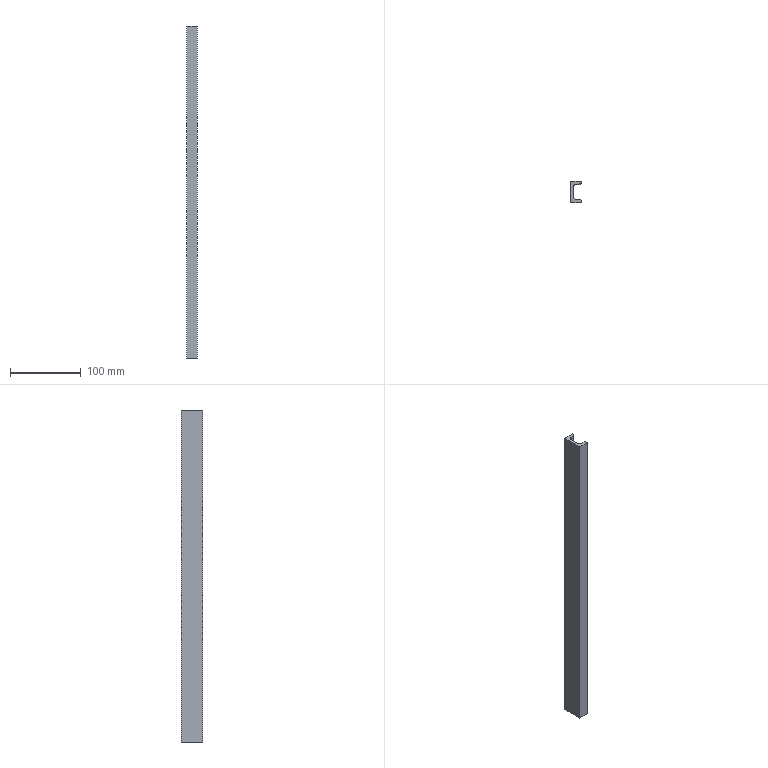Part | STEP file | DIN 1026-1 U 30x15 1785507675323 | 1 solid | 14 faces | box 15 x 30 x 470 mm | volume 103990 mm3 | plane 10 | cylinder 4 | commonest cylinder face diameters 4 x2 9 x2
STEP:
#1=CARTESIAN_POINT('',(4.,-6.066,485.));
#2=VERTEX_POINT('',#1);
#3=CARTESIAN_POINT('',(8.141,-10.551,485.));
#4=VERTEX_POINT('',#3);
#5=CARTESIAN_POINT('',(8.5,-6.066,485.));
#6=DIRECTION('',(0.,0.,1.));
#7=DIRECTION('',(-1.,0.,0.));
#8=AXIS2_PLACEMENT_3D('',#5,#6,#7);
#9=CIRCLE('',#8,4.5);
#10=EDGE_CURVE('',#2,#4,#9,.T.);
#11=ORIENTED_EDGE('',*,*,#10,.T.);
#12=CARTESIAN_POINT('',(8.141,-10.551,15.));
#13=VERTEX_POINT('',#12);
#14=CARTESIAN_POINT('',(8.141,-10.551,0.));
#15=DIRECTION('',(0.,0.,1.));
#16=VECTOR('',#15,10.);
#17=LINE('',#14,#16);
#18=EDGE_CURVE('',#13,#4,#17,.T.);
#19=ORIENTED_EDGE('',*,*,#18,.F.);
#20=CARTESIAN_POINT('',(4.,-6.066,15.));
#21=VERTEX_POINT('',#20);
#22=CARTESIAN_POINT('',(8.5,-6.066,15.));
#23=DIRECTION('',(0.,0.,1.));
#24=DIRECTION('',(-1.,0.,0.));
#25=AXIS2_PLACEMENT_3D('',#22,#23,#24);
#26=CIRCLE('',#25,4.5);
#27=EDGE_CURVE('',#21,#13,#26,.T.);
#28=ORIENTED_EDGE('',*,*,#27,.F.);
#29=CARTESIAN_POINT('',(4.,-6.066,0.));
#30=DIRECTION('',(0.,0.,1.));
#31=VECTOR('',#30,10.);
#32=LINE('',#29,#31);
#33=EDGE_CURVE('',#21,#2,#32,.T.);
#34=ORIENTED_EDGE('',*,*,#33,.T.);
#35=EDGE_LOOP('',(#11,#19,#28,#34));
#36=FACE_OUTER_BOUND('',#35,.T.);
#37=CARTESIAN_POINT('',(8.5,-6.066,0.));
#38=DIRECTION('',(0.,0.,1.));
#39=DIRECTION('',(-1.,0.,0.));
#40=AXIS2_PLACEMENT_3D('',#37,#38,#39);
#41=CYLINDRICAL_SURFACE('',#40,4.5);
#42=ADVANCED_FACE('',(#36),#41,.F.);
#43=CARTESIAN_POINT('',(13.159,-10.953,485.));
#44=VERTEX_POINT('',#43);
#45=CARTESIAN_POINT('',(7.403,-10.492,485.));
#46=DIRECTION('',(0.9968,-0.07975,0.));
#47=VECTOR('',#46,10.);
#48=LINE('',#45,#47);
#49=EDGE_CURVE('',#4,#44,#48,.T.);
#50=ORIENTED_EDGE('',*,*,#49,.T.);
#51=CARTESIAN_POINT('',(13.159,-10.953,15.));
#52=VERTEX_POINT('',#51);
#53=CARTESIAN_POINT('',(13.159,-10.953,0.));
#54=DIRECTION('',(0.,0.,1.));
#55=VECTOR('',#54,10.);
#56=LINE('',#53,#55);
#57=EDGE_CURVE('',#52,#44,#56,.T.);
#58=ORIENTED_EDGE('',*,*,#57,.F.);
#59=CARTESIAN_POINT('',(7.403,-10.492,15.));
#60=DIRECTION('',(0.9968,-0.07975,0.));
#61=VECTOR('',#60,10.);
#62=LINE('',#59,#61);
#63=EDGE_CURVE('',#13,#52,#62,.T.);
#64=ORIENTED_EDGE('',*,*,#63,.F.);
#65=ORIENTED_EDGE('',*,*,#18,.T.);
#66=EDGE_LOOP('',(#50,#58,#64,#65));
#67=FACE_OUTER_BOUND('',#66,.T.);
#68=CARTESIAN_POINT('',(8.141,-10.551,0.));
#69=DIRECTION('',(0.07975,0.9968,0.));
#70=DIRECTION('',(0.,0.,1.));
#71=AXIS2_PLACEMENT_3D('',#68,#69,#70);
#72=PLANE('',#71);
#73=ADVANCED_FACE('',(#67),#72,.T.);
#74=CARTESIAN_POINT('',(15.,-12.946,485.));
#75=VERTEX_POINT('',#74);
#76=CARTESIAN_POINT('',(13.,-12.946,485.));
#77=DIRECTION('',(0.,0.,-1.));
#78=DIRECTION('',(-1.,0.,0.));
#79=AXIS2_PLACEMENT_3D('',#76,#77,#78);
#80=CIRCLE('',#79,2.);
#81=EDGE_CURVE('',#44,#75,#80,.T.);
#82=ORIENTED_EDGE('',*,*,#81,.T.);
#83=CARTESIAN_POINT('',(15.,-12.946,15.));
#84=VERTEX_POINT('',#83);
#85=CARTESIAN_POINT('',(15.,-12.946,0.));
#86=DIRECTION('',(0.,0.,1.));
#87=VECTOR('',#86,10.);
#88=LINE('',#85,#87);
#89=EDGE_CURVE('',#84,#75,#88,.T.);
#90=ORIENTED_EDGE('',*,*,#89,.F.);
#91=CARTESIAN_POINT('',(13.,-12.946,15.));
#92=DIRECTION('',(0.,0.,-1.));
#93=DIRECTION('',(-1.,0.,0.));
#94=AXIS2_PLACEMENT_3D('',#91,#92,#93);
#95=CIRCLE('',#94,2.);
#96=EDGE_CURVE('',#52,#84,#95,.T.);
#97=ORIENTED_EDGE('',*,*,#96,.F.);
#98=ORIENTED_EDGE('',*,*,#57,.T.);
#99=EDGE_LOOP('',(#82,#90,#97,#98));
#100=FACE_OUTER_BOUND('',#99,.T.);
#101=CARTESIAN_POINT('',(13.,-12.946,0.));
#102=DIRECTION('',(0.,0.,1.));
#103=DIRECTION('',(-1.,0.,0.));
#104=AXIS2_PLACEMENT_3D('',#101,#102,#103);
#105=CYLINDRICAL_SURFACE('',#104,2.);
#106=ADVANCED_FACE('',(#100),#105,.T.);
#107=CARTESIAN_POINT('',(15.,-15.,485.));
#108=VERTEX_POINT('',#107);
#109=CARTESIAN_POINT('',(15.,-6.473,485.));
#110=DIRECTION('',(0.,-1.,0.));
#111=VECTOR('',#110,10.);
#112=LINE('',#109,#111);
#113=EDGE_CURVE('',#75,#108,#112,.T.);
#114=ORIENTED_EDGE('',*,*,#113,.T.);
#115=CARTESIAN_POINT('',(15.,-15.,15.));
#116=VERTEX_POINT('',#115);
#117=CARTESIAN_POINT('',(15.,-15.,0.));
#118=DIRECTION('',(0.,0.,1.));
#119=VECTOR('',#118,10.);
#120=LINE('',#117,#119);
#121=EDGE_CURVE('',#116,#108,#120,.T.);
#122=ORIENTED_EDGE('',*,*,#121,.F.);
#123=CARTESIAN_POINT('',(15.,-6.473,15.));
#124=DIRECTION('',(0.,-1.,0.));
#125=VECTOR('',#124,10.);
#126=LINE('',#123,#125);
#127=EDGE_CURVE('',#84,#116,#126,.T.);
#128=ORIENTED_EDGE('',*,*,#127,.F.);
#129=ORIENTED_EDGE('',*,*,#89,.T.);
#130=EDGE_LOOP('',(#114,#122,#128,#129));
#131=FACE_OUTER_BOUND('',#130,.T.);
#132=CARTESIAN_POINT('',(15.,-12.946,0.));
#133=DIRECTION('',(1.,0.,0.));
#134=DIRECTION('',(0.,0.,-1.));
#135=AXIS2_PLACEMENT_3D('',#132,#133,#134);
#136=PLANE('',#135);
#137=ADVANCED_FACE('',(#131),#136,.T.);
#138=CARTESIAN_POINT('',(0.,-15.,485.));
#139=VERTEX_POINT('',#138);
#140=CARTESIAN_POINT('',(11.25,-15.,485.));
#141=DIRECTION('',(-1.,0.,0.));
#142=VECTOR('',#141,10.);
#143=LINE('',#140,#142);
#144=EDGE_CURVE('',#108,#139,#143,.T.);
#145=ORIENTED_EDGE('',*,*,#144,.T.);
#146=CARTESIAN_POINT('',(0.,-15.,15.));
#147=VERTEX_POINT('',#146);
#148=CARTESIAN_POINT('',(0.,-15.,0.));
#149=DIRECTION('',(0.,0.,1.));
#150=VECTOR('',#149,10.);
#151=LINE('',#148,#150);
#152=EDGE_CURVE('',#147,#139,#151,.T.);
#153=ORIENTED_EDGE('',*,*,#152,.F.);
#154=CARTESIAN_POINT('',(11.25,-15.,15.));
#155=DIRECTION('',(-1.,0.,0.));
#156=VECTOR('',#155,10.);
#157=LINE('',#154,#156);
#158=EDGE_CURVE('',#116,#147,#157,.T.);
#159=ORIENTED_EDGE('',*,*,#158,.F.);
#160=ORIENTED_EDGE('',*,*,#121,.T.);
#161=EDGE_LOOP('',(#145,#153,#159,#160));
#162=FACE_OUTER_BOUND('',#161,.T.);
#163=CARTESIAN_POINT('',(15.,-15.,0.));
#164=DIRECTION('',(0.,-1.,0.));
#165=DIRECTION('',(0.,0.,-1.));
#166=AXIS2_PLACEMENT_3D('',#163,#164,#165);
#167=PLANE('',#166);
#168=ADVANCED_FACE('',(#162),#167,.T.);
#169=CARTESIAN_POINT('',(0.,15.,485.));
#170=VERTEX_POINT('',#169);
#171=CARTESIAN_POINT('',(0.,0.,485.));
#172=DIRECTION('',(0.,1.,0.));
#173=VECTOR('',#172,10.);
#174=LINE('',#171,#173);
#175=EDGE_CURVE('',#139,#170,#174,.T.);
#176=ORIENTED_EDGE('',*,*,#175,.T.);
#177=CARTESIAN_POINT('',(0.,15.,15.));
#178=VERTEX_POINT('',#177);
#179=CARTESIAN_POINT('',(0.,15.,0.));
#180=DIRECTION('',(0.,0.,1.));
#181=VECTOR('',#180,10.);
#182=LINE('',#179,#181);
#183=EDGE_CURVE('',#178,#170,#182,.T.);
#184=ORIENTED_EDGE('',*,*,#183,.F.);
#185=CARTESIAN_POINT('',(0.,0.,15.));
#186=DIRECTION('',(0.,1.,0.));
#187=VECTOR('',#186,10.);
#188=LINE('',#185,#187);
#189=EDGE_CURVE('',#147,#178,#188,.T.);
#190=ORIENTED_EDGE('',*,*,#189,.F.);
#191=ORIENTED_EDGE('',*,*,#152,.T.);
#192=EDGE_LOOP('',(#176,#184,#190,#191));
#193=FACE_OUTER_BOUND('',#192,.T.);
#194=CARTESIAN_POINT('',(0.,0.,0.));
#195=DIRECTION('',(-1.,0.,0.));
#196=DIRECTION('',(0.,0.,1.));
#197=AXIS2_PLACEMENT_3D('',#194,#195,#196);
#198=PLANE('',#197);
#199=ADVANCED_FACE('',(#193),#198,.T.);
#200=CARTESIAN_POINT('',(15.,15.,485.));
#201=VERTEX_POINT('',#200);
#202=CARTESIAN_POINT('',(3.75,15.,485.));
#203=DIRECTION('',(1.,0.,0.));
#204=VECTOR('',#203,10.);
#205=LINE('',#202,#204);
#206=EDGE_CURVE('',#170,#201,#205,.T.);
#207=ORIENTED_EDGE('',*,*,#206,.T.);
#208=CARTESIAN_POINT('',(15.,15.,15.));
#209=VERTEX_POINT('',#208);
#210=CARTESIAN_POINT('',(15.,15.,0.));
#211=DIRECTION('',(0.,0.,1.));
#212=VECTOR('',#211,10.);
#213=LINE('',#210,#212);
#214=EDGE_CURVE('',#209,#201,#213,.T.);
#215=ORIENTED_EDGE('',*,*,#214,.F.);
#216=CARTESIAN_POINT('',(3.75,15.,15.));
#217=DIRECTION('',(1.,0.,0.));
#218=VECTOR('',#217,10.);
#219=LINE('',#216,#218);
#220=EDGE_CURVE('',#178,#209,#219,.T.);
#221=ORIENTED_EDGE('',*,*,#220,.F.);
#222=ORIENTED_EDGE('',*,*,#183,.T.);
#223=EDGE_LOOP('',(#207,#215,#221,#222));
#224=FACE_OUTER_BOUND('',#223,.T.);
#225=CARTESIAN_POINT('',(0.,15.,0.));
#226=DIRECTION('',(0.,1.,0.));
#227=DIRECTION('',(0.,0.,1.));
#228=AXIS2_PLACEMENT_3D('',#225,#226,#227);
#229=PLANE('',#228);
#230=ADVANCED_FACE('',(#224),#229,.T.);
#231=CARTESIAN_POINT('',(15.,12.946,485.));
#232=VERTEX_POINT('',#231);
#233=CARTESIAN_POINT('',(15.,7.5,485.));
#234=DIRECTION('',(0.,-1.,0.));
#235=VECTOR('',#234,10.);
#236=LINE('',#233,#235);
#237=EDGE_CURVE('',#201,#232,#236,.T.);
#238=ORIENTED_EDGE('',*,*,#237,.T.);
#239=CARTESIAN_POINT('',(15.,12.946,15.));
#240=VERTEX_POINT('',#239);
#241=CARTESIAN_POINT('',(15.,12.946,0.));
#242=DIRECTION('',(0.,0.,1.));
#243=VECTOR('',#242,10.);
#244=LINE('',#241,#243);
#245=EDGE_CURVE('',#240,#232,#244,.T.);
#246=ORIENTED_EDGE('',*,*,#245,.F.);
#247=CARTESIAN_POINT('',(15.,7.5,15.));
#248=DIRECTION('',(0.,-1.,0.));
#249=VECTOR('',#248,10.);
#250=LINE('',#247,#249);
#251=EDGE_CURVE('',#209,#240,#250,.T.);
#252=ORIENTED_EDGE('',*,*,#251,.F.);
#253=ORIENTED_EDGE('',*,*,#214,.T.);
#254=EDGE_LOOP('',(#238,#246,#252,#253));
#255=FACE_OUTER_BOUND('',#254,.T.);
#256=CARTESIAN_POINT('',(15.,15.,0.));
#257=DIRECTION('',(1.,0.,0.));
#258=DIRECTION('',(0.,0.,-1.));
#259=AXIS2_PLACEMENT_3D('',#256,#257,#258);
#260=PLANE('',#259);
#261=ADVANCED_FACE('',(#255),#260,.T.);
#262=CARTESIAN_POINT('',(13.159,10.953,485.));
#263=VERTEX_POINT('',#262);
#264=CARTESIAN_POINT('',(13.,12.946,485.));
#265=DIRECTION('',(0.,0.,-1.));
#266=DIRECTION('',(-0.07975,0.9968,0.));
#267=AXIS2_PLACEMENT_3D('',#264,#265,#266);
#268=CIRCLE('',#267,2.);
#269=EDGE_CURVE('',#232,#263,#268,.T.);
#270=ORIENTED_EDGE('',*,*,#269,.T.);
#271=CARTESIAN_POINT('',(13.159,10.953,15.));
#272=VERTEX_POINT('',#271);
#273=CARTESIAN_POINT('',(13.159,10.953,0.));
#274=DIRECTION('',(0.,0.,1.));
#275=VECTOR('',#274,10.);
#276=LINE('',#273,#275);
#277=EDGE_CURVE('',#272,#263,#276,.T.);
#278=ORIENTED_EDGE('',*,*,#277,.F.);
#279=CARTESIAN_POINT('',(13.,12.946,15.));
#280=DIRECTION('',(0.,0.,-1.));
#281=DIRECTION('',(-0.07975,0.9968,0.));
#282=AXIS2_PLACEMENT_3D('',#279,#280,#281);
#283=CIRCLE('',#282,2.);
#284=EDGE_CURVE('',#240,#272,#283,.T.);
#285=ORIENTED_EDGE('',*,*,#284,.F.);
#286=ORIENTED_EDGE('',*,*,#245,.T.);
#287=EDGE_LOOP('',(#270,#278,#285,#286));
#288=FACE_OUTER_BOUND('',#287,.T.);
#289=CARTESIAN_POINT('',(13.,12.946,0.));
#290=DIRECTION('',(0.,0.,1.));
#291=DIRECTION('',(-0.07975,0.9968,0.));
#292=AXIS2_PLACEMENT_3D('',#289,#290,#291);
#293=CYLINDRICAL_SURFACE('',#292,2.);
#294=ADVANCED_FACE('',(#288),#293,.T.);
#295=CARTESIAN_POINT('',(8.141,10.551,485.));
#296=VERTEX_POINT('',#295);
#297=CARTESIAN_POINT('',(9.912,10.693,485.));
#298=DIRECTION('',(-0.9968,-0.07975,0.));
#299=VECTOR('',#298,10.);
#300=LINE('',#297,#299);
#301=EDGE_CURVE('',#263,#296,#300,.T.);
#302=ORIENTED_EDGE('',*,*,#301,.T.);
#303=CARTESIAN_POINT('',(8.141,10.551,15.));
#304=VERTEX_POINT('',#303);
#305=CARTESIAN_POINT('',(8.141,10.551,0.));
#306=DIRECTION('',(0.,0.,1.));
#307=VECTOR('',#306,10.);
#308=LINE('',#305,#307);
#309=EDGE_CURVE('',#304,#296,#308,.T.);
#310=ORIENTED_EDGE('',*,*,#309,.F.);
#311=CARTESIAN_POINT('',(9.912,10.693,15.));
#312=DIRECTION('',(-0.9968,-0.07975,0.));
#313=VECTOR('',#312,10.);
#314=LINE('',#311,#313);
#315=EDGE_CURVE('',#272,#304,#314,.T.);
#316=ORIENTED_EDGE('',*,*,#315,.F.);
#317=ORIENTED_EDGE('',*,*,#277,.T.);
#318=EDGE_LOOP('',(#302,#310,#316,#317));
#319=FACE_OUTER_BOUND('',#318,.T.);
#320=CARTESIAN_POINT('',(13.159,10.953,0.));
#321=DIRECTION('',(0.07975,-0.9968,0.));
#322=DIRECTION('',(0.,0.,-1.));
#323=AXIS2_PLACEMENT_3D('',#320,#321,#322);
#324=PLANE('',#323);
#325=ADVANCED_FACE('',(#319),#324,.T.);
#326=CARTESIAN_POINT('',(4.,6.066,485.));
#327=VERTEX_POINT('',#326);
#328=CARTESIAN_POINT('',(8.5,6.066,485.));
#329=DIRECTION('',(0.,0.,1.));
#330=DIRECTION('',(-0.07975,0.9968,0.));
#331=AXIS2_PLACEMENT_3D('',#328,#329,#330);
#332=CIRCLE('',#331,4.5);
#333=EDGE_CURVE('',#296,#327,#332,.T.);
#334=ORIENTED_EDGE('',*,*,#333,.T.);
#335=CARTESIAN_POINT('',(4.,6.066,15.));
#336=VERTEX_POINT('',#335);
#337=CARTESIAN_POINT('',(4.,6.066,0.));
#338=DIRECTION('',(0.,0.,1.));
#339=VECTOR('',#338,10.);
#340=LINE('',#337,#339);
#341=EDGE_CURVE('',#336,#327,#340,.T.);
#342=ORIENTED_EDGE('',*,*,#341,.F.);
#343=CARTESIAN_POINT('',(8.5,6.066,15.));
#344=DIRECTION('',(0.,0.,1.));
#345=DIRECTION('',(-0.07975,0.9968,0.));
#346=AXIS2_PLACEMENT_3D('',#343,#344,#345);
#347=CIRCLE('',#346,4.5);
#348=EDGE_CURVE('',#304,#336,#347,.T.);
#349=ORIENTED_EDGE('',*,*,#348,.F.);
#350=ORIENTED_EDGE('',*,*,#309,.T.);
#351=EDGE_LOOP('',(#334,#342,#349,#350));
#352=FACE_OUTER_BOUND('',#351,.T.);
#353=CARTESIAN_POINT('',(8.5,6.066,0.));
#354=DIRECTION('',(0.,0.,1.));
#355=DIRECTION('',(-0.07975,0.9968,0.));
#356=AXIS2_PLACEMENT_3D('',#353,#354,#355);
#357=CYLINDRICAL_SURFACE('',#356,4.5);
#358=ADVANCED_FACE('',(#352),#357,.F.);
#359=CARTESIAN_POINT('',(4.,0.,485.));
#360=DIRECTION('',(0.,-1.,0.));
#361=VECTOR('',#360,10.);
#362=LINE('',#359,#361);
#363=EDGE_CURVE('',#327,#2,#362,.T.);
#364=ORIENTED_EDGE('',*,*,#363,.T.);
#365=ORIENTED_EDGE('',*,*,#33,.F.);
#366=CARTESIAN_POINT('',(4.,0.,15.));
#367=DIRECTION('',(0.,-1.,0.));
#368=VECTOR('',#367,10.);
#369=LINE('',#366,#368);
#370=EDGE_CURVE('',#336,#21,#369,.T.);
#371=ORIENTED_EDGE('',*,*,#370,.F.);
#372=ORIENTED_EDGE('',*,*,#341,.T.);
#373=EDGE_LOOP('',(#364,#365,#371,#372));
#374=FACE_OUTER_BOUND('',#373,.T.);
#375=CARTESIAN_POINT('',(4.,0.,0.));
#376=DIRECTION('',(1.,0.,0.));
#377=DIRECTION('',(0.,0.,-1.));
#378=AXIS2_PLACEMENT_3D('',#375,#376,#377);
#379=PLANE('',#378);
#380=ADVANCED_FACE('',(#374),#379,.T.);
#381=ORIENTED_EDGE('',*,*,#220,.T.);
#382=ORIENTED_EDGE('',*,*,#251,.T.);
#383=ORIENTED_EDGE('',*,*,#284,.T.);
#384=ORIENTED_EDGE('',*,*,#315,.T.);
#385=ORIENTED_EDGE('',*,*,#348,.T.);
#386=ORIENTED_EDGE('',*,*,#370,.T.);
#387=ORIENTED_EDGE('',*,*,#27,.T.);
#388=ORIENTED_EDGE('',*,*,#63,.T.);
#389=ORIENTED_EDGE('',*,*,#96,.T.);
#390=ORIENTED_EDGE('',*,*,#127,.T.);
#391=ORIENTED_EDGE('',*,*,#158,.T.);
#392=ORIENTED_EDGE('',*,*,#189,.T.);
#393=EDGE_LOOP('',(#381,#382,#383,#384,#385,#386,#387,#388,#389,#390,#391,#392));
#394=FACE_OUTER_BOUND('',#393,.T.);
#395=CARTESIAN_POINT('',(7.5,0.,15.));
#396=DIRECTION('',(0.,0.,1.));
#397=DIRECTION('',(1.,0.,0.));
#398=AXIS2_PLACEMENT_3D('',#395,#396,#397);
#399=PLANE('',#398);
#400=ADVANCED_FACE('',(#394),#399,.F.);
#401=ORIENTED_EDGE('',*,*,#206,.F.);
#402=ORIENTED_EDGE('',*,*,#175,.F.);
#403=ORIENTED_EDGE('',*,*,#144,.F.);
#404=ORIENTED_EDGE('',*,*,#113,.F.);
#405=ORIENTED_EDGE('',*,*,#81,.F.);
#406=ORIENTED_EDGE('',*,*,#49,.F.);
#407=ORIENTED_EDGE('',*,*,#10,.F.);
#408=ORIENTED_EDGE('',*,*,#363,.F.);
#409=ORIENTED_EDGE('',*,*,#333,.F.);
#410=ORIENTED_EDGE('',*,*,#301,.F.);
#411=ORIENTED_EDGE('',*,*,#269,.F.);
#412=ORIENTED_EDGE('',*,*,#237,.F.);
#413=EDGE_LOOP('',(#401,#402,#403,#404,#405,#406,#407,#408,#409,#410,#411,#412));
#414=FACE_OUTER_BOUND('',#413,.T.);
#415=CARTESIAN_POINT('',(7.5,0.,485.));
#416=DIRECTION('',(0.,0.,1.));
#417=DIRECTION('',(1.,0.,0.));
#418=AXIS2_PLACEMENT_3D('',#415,#416,#417);
#419=PLANE('',#418);
#420=ADVANCED_FACE('',(#414),#419,.T.);
#421=CLOSED_SHELL('',(#42,#73,#106,#137,#168,#199,#230,#261,#294,#325,#358,#380,#400,#420));
#422=MANIFOLD_SOLID_BREP('',#421);
#423=(LENGTH_UNIT()NAMED_UNIT(*)SI_UNIT(.MILLI.,.METRE.));
#424=UNCERTAINTY_MEASURE_WITH_UNIT(LENGTH_MEASURE(0.01),#423,'','');
#425=(NAMED_UNIT(*)PLANE_ANGLE_UNIT()SI_UNIT($,.RADIAN.));
#426=(NAMED_UNIT(*)SI_UNIT($,.STERADIAN.)SOLID_ANGLE_UNIT());
#427=(GEOMETRIC_REPRESENTATION_CONTEXT(3)GLOBAL_UNCERTAINTY_ASSIGNED_CONTEXT((#424))GLOBAL_UNIT_ASSIGNED_CONTEXT((#423,#425,#426))REPRESENTATION_CONTEXT('',''));
#428=ADVANCED_BREP_SHAPE_REPRESENTATION('',(#422),#427);